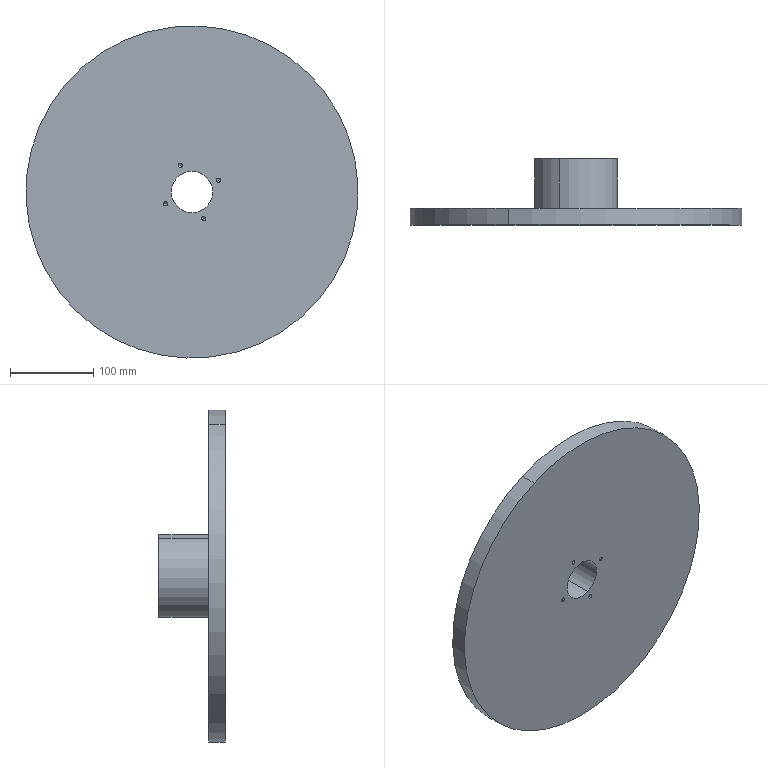Part | STEP file | M6 threaded hole 1-1 | 1 solid | 113 faces | box 400 x 80 x 400 mm | volume 2816788 mm3 | cylinder 70 | plane 27 | cone 16 | commonest cylinder face diameters 6.6 x48 5 x16 50 x2 100 x2 400 x2